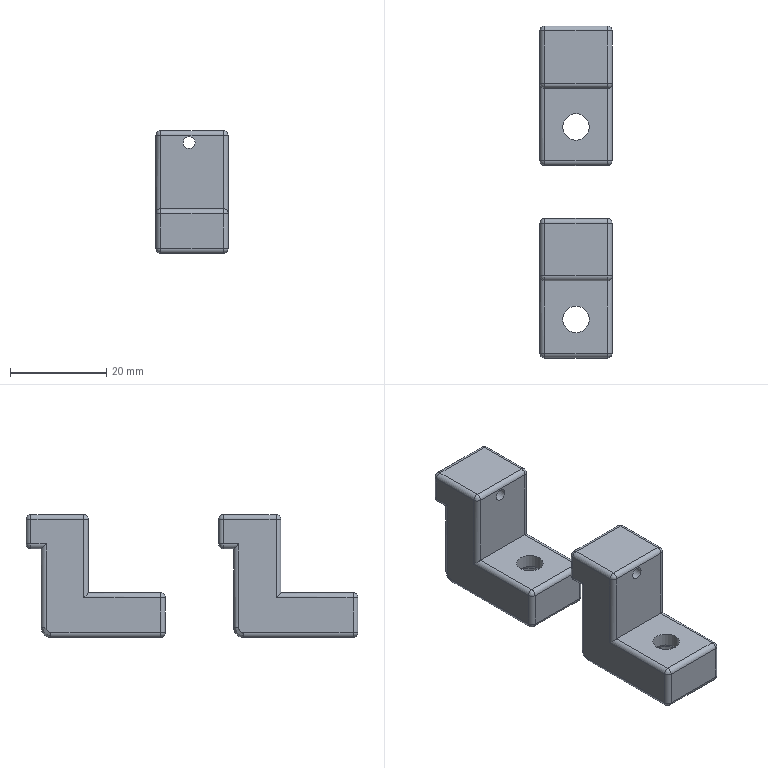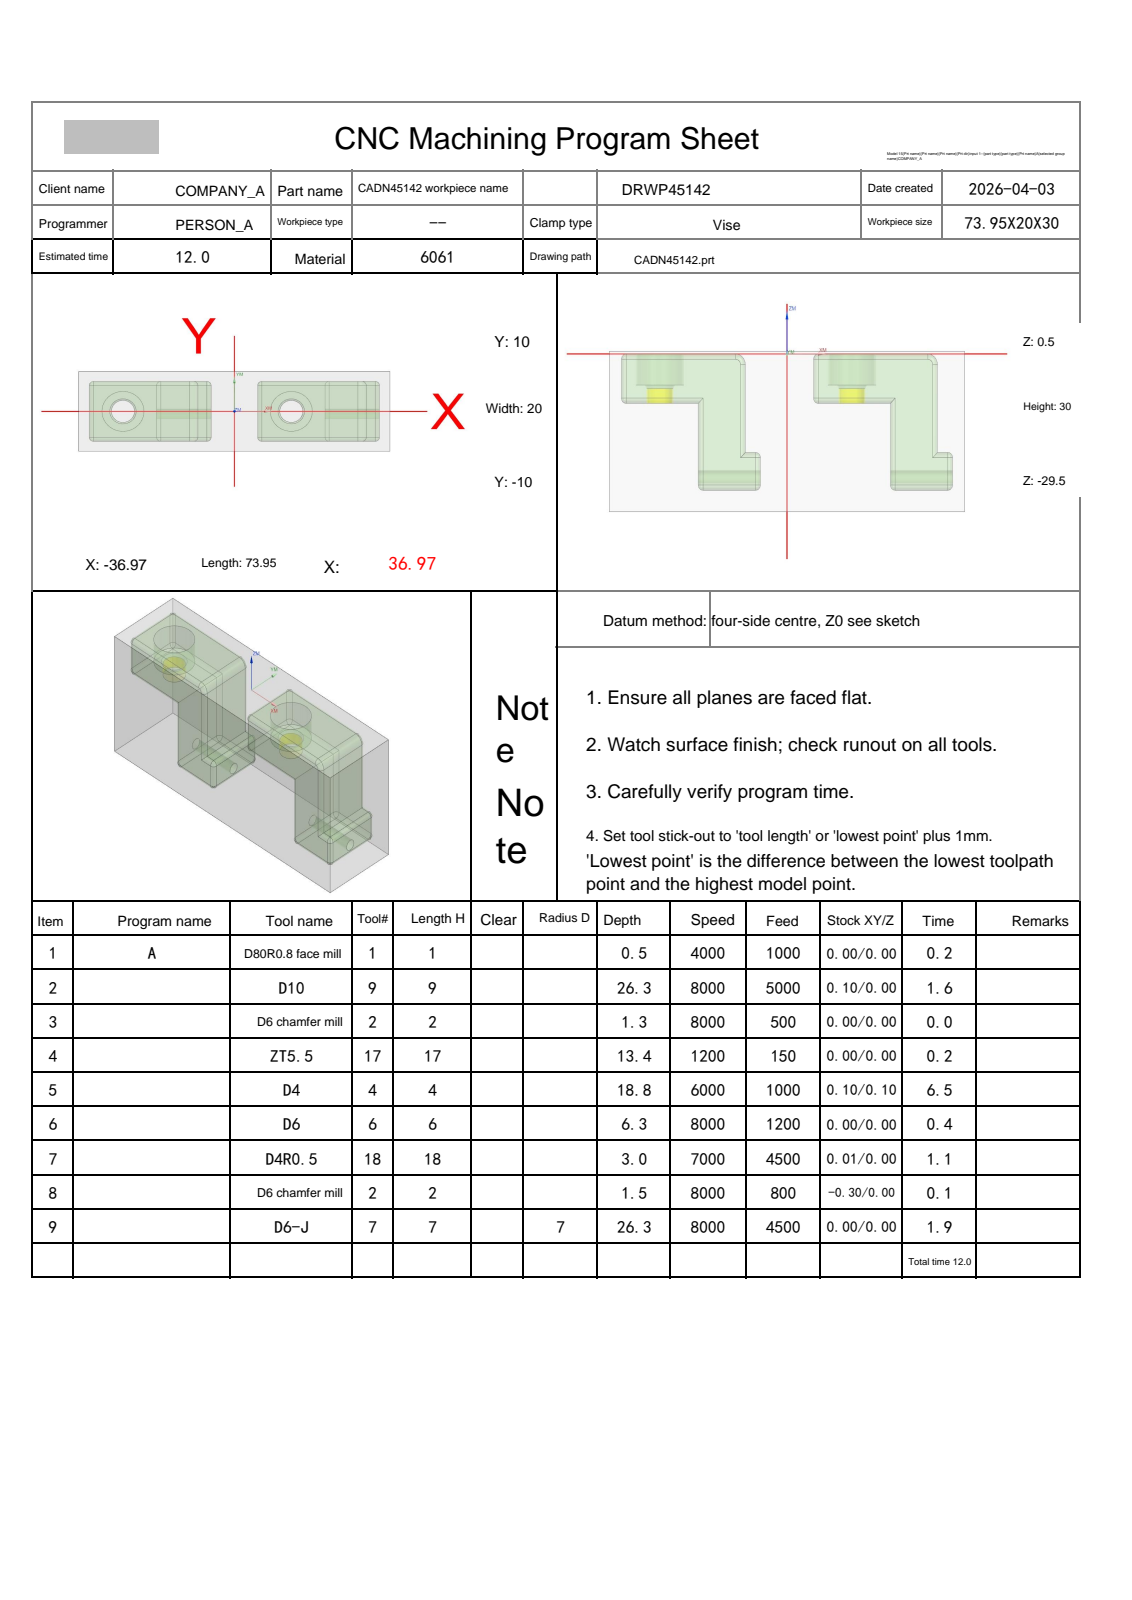NC program | NX | posted by the shop | part box 15 x 68.95 x 25.5 mm
Lines 1 to 3214 of 6074, first 2006 of 3212 lines:
%
O0001
(Machine time: 13.80 MIN)
(===Total Tool:8===)
(T1=D80R0.8 face mill D=80.  R=0.8  D-  H01 Z=-0.   )
(T9=D10     D=10.  R=0.   D-  H09 Z=-25.8 )
(T2=D6 chamfer mill   D=6.   R=0.   D-  H02 Z=-1.   )
(T17=ZT5.5  D=5.5  DR_a=118 D-  H17 Z=-12.9 )
(T4=D4      D=4.   R=0.   D-  H04 Z=-18.31)
(T6=D6      D=6.   R=0.   D6  H06 Z=-5.8  )
(T18=D4R0.5 D=4.   R=0.5  D-  H18 Z=-2.5  )
(T7=D6-J    D=6.   R=0.   D7  H07 Z=-25.8 )
G80 G90 G17 G49 G40
G91 G28 Z0
M01
N1 T01 M06
(D80R0.8 face mill D=80. R=0.8 H=01 ce=0.00 di=0.00)
G00 G90 G54 X-79.475 Y0.0 M03 S4000
G43 H01 Z20.
M08
Z2.
G01 Z0.0 F1000.
X-74.475
X74.475
X79.475
Z2.
G00 Z20.
G91 G28 Z0.0
M05
M09
G91 G28 Z0.0
M01
N2 T09 M06
(D10  D=10. R=0. H=09 ce=0.10 di=0.00)
G00 G90 G54 X20. Y-12.6 M03 S8000
G43 H09 Z20.
M08
Z.5
G01 X6.525 Z.409 F5000.
G02 X.425 Y-6.5 Z.345 I0.0 J6.1
G01 Y6.5 Z.257
G02 X6.525 Y12.6 Z.192 I6.1 J0.0
G01 X33.475 Z.011
G02 X39.575 Y6.5 Z-.054 I0.0 J-6.1
G01 Y-6.5 Z-.142
G02 X33.475 Y-12.6 Z-.206 I-6.1 J0.0
G01 X6.525 Z-.388
G02 X.425 Y-6.5 Z-.452 I0.0 J6.1
G01 Y6.5 Z-.54
G02 X6.525 Y12.6 Z-.605 I6.1 J0.0
G01 X33.475 Z-.786
G02 X39.575 Y6.5 Z-.851 I0.0 J-6.1
G01 Y-6.5 Z-.939
G02 X33.475 Y-12.6 Z-1.003 I-6.1 J0.0
G01 X6.525 Z-1.185
G02 X.425 Y-6.5 Z-1.249 I0.0 J6.1
G01 Y6.5 Z-1.337
G02 X6.525 Y12.6 Z-1.402 I6.1 J0.0
G01 X33.475 Z-1.583
G02 X39.575 Y6.5 Z-1.648 I0.0 J-6.1
G01 Y-6.5 Z-1.735
G02 X33.475 Y-12.6 Z-1.8 I-6.1 J0.0
G01 X6.525 Z-1.982
G02 X.425 Y-6.5 Z-2.046 I0.0 J6.1
G01 Y6.5 Z-2.134
G02 X6.525 Y12.6 Z-2.199 I6.1 J0.0
G01 X33.475 Z-2.38
G02 X39.575 Y6.5 Z-2.445 I0.0 J-6.1
G01 Y-6.5 Z-2.532
G02 X33.475 Y-12.6 Z-2.597 I-6.1 J0.0
G01 X6.525 Z-2.779
G02 X.425 Y-6.5 Z-2.843 I0.0 J6.1
G01 Y6.5 Z-2.931
G02 X6.525 Y12.6 Z-2.996 I6.1 J0.0
G01 X33.475 Z-3.177
G02 X39.575 Y6.5 Z-3.242 I0.0 J-6.1
G01 Y-6.5 Z-3.329
G02 X33.475 Y-12.6 Z-3.394 I-6.1 J0.0
G01 X6.525 Z-3.576
G02 X.425 Y-6.5 Z-3.64 I0.0 J6.1
G01 Y6.5 Z-3.728
G02 X6.525 Y12.6 Z-3.793 I6.1 J0.0
G01 X33.475 Z-3.974
G02 X39.575 Y6.5 Z-4.039 I0.0 J-6.1
G01 Y-6.5 Z-4.126
G02 X33.475 Y-12.6 Z-4.191 I-6.1 J0.0
G01 X6.525 Z-4.373
G02 X.425 Y-6.5 Z-4.437 I0.0 J6.1
G01 Y6.5 Z-4.525
G02 X6.525 Y12.6 Z-4.589 I6.1 J0.0
G01 X33.475 Z-4.771
G02 X39.575 Y6.5 Z-4.836 I0.0 J-6.1
G01 Y-6.5 Z-4.923
G02 X33.475 Y-12.6 Z-4.988 I-6.1 J0.0
G01 X6.525 Z-5.17
G02 X.425 Y-6.5 Z-5.234 I0.0 J6.1
G01 Y6.5 Z-5.322
G02 X6.525 Y12.6 Z-5.386 I6.1 J0.0
G01 X33.475 Z-5.568
G02 X39.575 Y6.5 Z-5.633 I0.0 J-6.1
G01 Y-6.5 Z-5.72
G02 X33.475 Y-12.6 Z-5.785 I-6.1 J0.0
G01 X6.525 Z-5.967
G02 X.425 Y-6.5 Z-6.031 I0.0 J6.1
G01 Y6.5 Z-6.119
G02 X6.525 Y12.6 Z-6.183 I6.1 J0.0
G01 X33.475 Z-6.365
G02 X39.575 Y6.5 Z-6.43 I0.0 J-6.1
G01 Y-6.5 Z-6.517
G02 X33.475 Y-12.6 Z-6.582 I-6.1 J0.0
G01 X6.525 Z-6.764
G02 X.425 Y-6.5 Z-6.828 I0.0 J6.1
G01 Y6.5 Z-6.916
G02 X6.525 Y12.6 Z-6.98 I6.1 J0.0
G01 X33.475 Z-7.162
G02 X39.575 Y6.5 Z-7.227 I0.0 J-6.1
G01 Y-6.5 Z-7.314
G02 X33.475 Y-12.6 Z-7.379 I-6.1 J0.0
G01 X6.525 Z-7.561
G02 X.425 Y-6.5 Z-7.625 I0.0 J6.1
G01 Y6.5 Z-7.713
G02 X6.525 Y12.6 Z-7.777 I6.1 J0.0
G01 X33.475 Z-7.959
G02 X39.575 Y6.5 Z-8.024 I0.0 J-6.1
G01 Y-6.5 Z-8.111
G02 X33.475 Y-12.6 Z-8.176 I-6.1 J0.0
G01 X6.525 Z-8.358
G02 X.425 Y-6.5 Z-8.422 I0.0 J6.1
G01 Y6.5 Z-8.51
G02 X6.525 Y12.6 Z-8.574 I6.1 J0.0
G01 X33.475 Z-8.756
G02 X39.575 Y6.5 Z-8.821 I0.0 J-6.1
G01 Y-6.5 Z-8.908
G02 X33.475 Y-12.6 Z-8.973 I-6.1 J0.0
G01 X6.525 Z-9.154
G02 X.425 Y-6.5 Z-9.219 I0.0 J6.1
G01 Y6.5 Z-9.307
G02 X6.525 Y12.6 Z-9.371 I6.1 J0.0
G01 X33.475 Z-9.553
G02 X39.575 Y6.5 Z-9.618 I0.0 J-6.1
G01 Y-6.5 Z-9.705
G02 X33.475 Y-12.6 Z-9.77 I-6.1 J0.0
G01 X6.525 Z-9.951
G02 X.425 Y-6.5 Z-10.016 I0.0 J6.1
G01 Y6.5 Z-10.104
G02 X6.525 Y12.6 Z-10.168 I6.1 J0.0
G01 X33.475 Z-10.35
G02 X39.575 Y6.5 Z-10.415 I0.0 J-6.1
G01 Y-6.5 Z-10.502
G02 X33.475 Y-12.6 Z-10.567 I-6.1 J0.0
G01 X6.525 Z-10.748
G02 X.425 Y-6.5 Z-10.813 I0.0 J6.1
G01 Y6.5 Z-10.901
G02 X6.525 Y12.6 Z-10.965 I6.1 J0.0
G01 X33.475 Z-11.147
G02 X39.575 Y6.5 Z-11.211 I0.0 J-6.1
G01 Y-6.5 Z-11.299
G02 X33.475 Y-12.6 Z-11.364 I-6.1 J0.0
G01 X6.525 Z-11.545
G02 X.425 Y-6.5 Z-11.61 I0.0 J6.1
G01 Y6.5 Z-11.698
G02 X6.525 Y12.6 Z-11.762 I6.1 J0.0
G01 X33.475 Z-11.944
G02 X39.575 Y6.5 Z-12.008 I0.0 J-6.1
G01 Y-6.5 Z-12.096
G02 X33.475 Y-12.6 Z-12.161 I-6.1 J0.0
G01 X6.525 Z-12.342
G02 X.425 Y-6.5 Z-12.407 I0.0 J6.1
G01 Y6.5 Z-12.495
G02 X6.525 Y12.6 Z-12.559 I6.1 J0.0
G01 X33.475 Z-12.741
G02 X39.575 Y6.5 Z-12.805 I0.0 J-6.1
G01 Y-6.5 Z-12.893
G02 X33.475 Y-12.6 Z-12.958 I-6.1 J0.0
G01 X6.525 Z-13.139
G02 X.425 Y-6.5 Z-13.204 I0.0 J6.1
G01 Y6.5 Z-13.292
G02 X6.525 Y12.6 Z-13.356 I6.1 J0.0
G01 X33.475 Z-13.538
G02 X39.575 Y6.5 Z-13.602 I0.0 J-6.1
G01 Y-6.5 Z-13.69
G02 X33.475 Y-12.6 Z-13.755 I-6.1 J0.0
G01 X6.525 Z-13.936
G02 X.425 Y-6.5 Z-14.001 I0.0 J6.1
G01 Y6.5 Z-14.089
G02 X6.525 Y12.6 Z-14.153 I6.1 J0.0
G01 X33.475 Z-14.335
G02 X39.575 Y6.5 Z-14.399 I0.0 J-6.1
G01 Y-6.5 Z-14.487
G02 X33.475 Y-12.6 Z-14.552 I-6.1 J0.0
G01 X6.525 Z-14.733
G02 X.425 Y-6.5 Z-14.798 I0.0 J6.1
G01 Y6.5 Z-14.885
G02 X6.525 Y12.6 Z-14.95 I6.1 J0.0
G01 X33.475 Z-15.132
G02 X39.575 Y6.5 Z-15.196 I0.0 J-6.1
G01 Y-6.5 Z-15.284
G02 X33.475 Y-12.6 Z-15.349 I-6.1 J0.0
G01 X6.525 Z-15.53
G02 X.425 Y-6.5 Z-15.595 I0.0 J6.1
G01 Y6.5 Z-15.682
G02 X6.525 Y12.6 Z-15.747 I6.1 J0.0
G01 X33.475 Z-15.929
G02 X39.575 Y6.5 Z-15.993 I0.0 J-6.1
G01 Y-6.5 Z-16.081
G02 X33.475 Y-12.6 Z-16.146 I-6.1 J0.0
G01 X6.525 Z-16.327
G02 X.425 Y-6.5 Z-16.392 I0.0 J6.1
G01 Y6.5 Z-16.479
G02 X6.525 Y12.6 Z-16.544 I6.1 J0.0
G01 X33.475 Z-16.726
G02 X39.575 Y6.5 Z-16.79 I0.0 J-6.1
G01 Y-6.5 Z-16.878
G02 X33.475 Y-12.6 Z-16.943 I-6.1 J0.0
G01 X6.525 Z-17.124
G02 X.425 Y-6.5 Z-17.189 I0.0 J6.1
G01 Y6.5 Z-17.276
G02 X6.525 Y12.6 Z-17.341 I6.1 J0.0
G01 X33.475 Z-17.523
G02 X39.575 Y6.5 Z-17.587 I0.0 J-6.1
G01 Y-6.5 Z-17.675
G02 X33.475 Y-12.6 Z-17.739 I-6.1 J0.0
G01 X6.525 Z-17.921
G02 X.425 Y-6.5 Z-17.986 I0.0 J6.1
G01 Y6.5 Z-18.073
G02 X6.525 Y12.6 Z-18.138 I6.1 J0.0
G01 X33.475 Z-18.32
G02 X39.575 Y6.5 Z-18.384 I0.0 J-6.1
G01 Y-6.5 Z-18.472
G02 X33.475 Y-12.6 Z-18.536 I-6.1 J0.0
G01 X6.525 Z-18.718
G02 X.425 Y-6.5 Z-18.783 I0.0 J6.1
G01 Y6.5 Z-18.87
G02 X6.525 Y12.6 Z-18.935 I6.1 J0.0
G01 X33.475 Z-19.117
G02 X39.575 Y6.5 Z-19.181 I0.0 J-6.1
G01 Y-6.5 Z-19.269
G02 X33.475 Y-12.6 Z-19.333 I-6.1 J0.0
G01 X6.525 Z-19.515
G02 X.425 Y-6.5 Z-19.58 I0.0 J6.1
G01 Y6.5 Z-19.667
G02 X6.525 Y12.6 Z-19.732 I6.1 J0.0
G01 X33.475 Z-19.914
G02 X39.575 Y6.5 Z-19.978 I0.0 J-6.1
G01 Y-6.5 Z-20.066
G02 X33.475 Y-12.6 Z-20.13 I-6.1 J0.0
G01 X6.525 Z-20.312
G02 X.425 Y-6.5 Z-20.377 I0.0 J6.1
G01 Y6.5 Z-20.464
G02 X6.525 Y12.6 Z-20.529 I6.1 J0.0
G01 X33.475 Z-20.711
G02 X39.575 Y6.5 Z-20.775 I0.0 J-6.1
G01 Y-6.5 Z-20.863
G02 X33.475 Y-12.6 Z-20.927 I-6.1 J0.0
G01 X6.525 Z-21.109
G02 X.425 Y-6.5 Z-21.174 I0.0 J6.1
G01 Y6.5 Z-21.261
G02 X6.525 Y12.6 Z-21.326 I6.1 J0.0
G01 X33.475 Z-21.508
G02 X39.575 Y6.5 Z-21.572 I0.0 J-6.1
G01 Y-6.5 Z-21.66
G02 X33.475 Y-12.6 Z-21.724 I-6.1 J0.0
G01 X6.525 Z-21.906
G02 X.425 Y-6.5 Z-21.971 I0.0 J6.1
G01 Y6.5 Z-22.058
G02 X6.525 Y12.6 Z-22.123 I6.1 J0.0
G01 X33.475 Z-22.304
G02 X39.575 Y6.5 Z-22.369 I0.0 J-6.1
G01 Y-6.5 Z-22.457
G02 X33.475 Y-12.6 Z-22.521 I-6.1 J0.0
G01 X6.525 Z-22.703
G02 X.425 Y-6.5 Z-22.768 I0.0 J6.1
G01 Y6.5 Z-22.855
G02 X6.525 Y12.6 Z-22.92 I6.1 J0.0
G01 X33.475 Z-23.101
G02 X39.575 Y6.5 Z-23.166 I0.0 J-6.1
G01 Y-6.5 Z-23.254
G02 X33.475 Y-12.6 Z-23.318 I-6.1 J0.0
G01 X6.525 Z-23.5
G02 X.425 Y-6.5 Z-23.565 I0.0 J6.1
G01 Y6.5 Z-23.652
G02 X6.525 Y12.6 Z-23.717 I6.1 J0.0
G01 X33.475 Z-23.898
G02 X39.575 Y6.5 Z-23.963 I0.0 J-6.1
G01 Y-6.5 Z-24.051
G02 X33.475 Y-12.6 Z-24.115 I-6.1 J0.0
G01 X6.525 Z-24.297
G02 X.425 Y-6.5 Z-24.361 I0.0 J6.1
G01 Y6.5 Z-24.449
G02 X6.525 Y12.6 Z-24.514 I6.1 J0.0
G01 X33.475 Z-24.695
G02 X39.575 Y6.5 Z-24.76 I0.0 J-6.1
G01 Y-6.5 Z-24.848
G02 X33.475 Y-12.6 Z-24.912 I-6.1 J0.0
G01 X6.525 Z-25.094
G02 X.425 Y-6.5 Z-25.158 I0.0 J6.1
G01 Y6.5 Z-25.246
G02 X6.525 Y12.6 Z-25.311 I6.1 J0.0
G01 X33.475 Z-25.492
G02 X39.575 Y6.5 Z-25.557 I0.0 J-6.1
G01 Y-6.5 Z-25.645
G02 X33.475 Y-12.6 Z-25.709 I-6.1 J0.0
G01 X20. Z-25.8
X6.525
G02 X.425 Y-6.5 I0.0 J6.1
G01 Y6.5
G02 X6.525 Y12.6 I6.1 J0.0
G01 X33.475
G02 X39.575 Y6.5 I0.0 J-6.1
G01 Y-6.5
G02 X33.475 Y-12.6 I-6.1 J0.0
G01 X20.
X19.5
Z-24.8
G00 Z20.
X-20.
Z.5
G01 X-33.475 Z.409
G02 X-39.575 Y-6.5 Z.345 I0.0 J6.1
G01 Y6.5 Z.257
G02 X-33.475 Y12.6 Z.192 I6.1 J0.0
G01 X-6.525 Z.011
G02 X-.425 Y6.5 Z-.054 I0.0 J-6.1
G01 Y-6.5 Z-.142
G02 X-6.525 Y-12.6 Z-.206 I-6.1 J0.0
G01 X-33.475 Z-.388
G02 X-39.575 Y-6.5 Z-.452 I0.0 J6.1
G01 Y6.5 Z-.54
G02 X-33.475 Y12.6 Z-.605 I6.1 J0.0
G01 X-6.525 Z-.786
G02 X-.425 Y6.5 Z-.851 I0.0 J-6.1
G01 Y-6.5 Z-.939
G02 X-6.525 Y-12.6 Z-1.003 I-6.1 J0.0
G01 X-33.475 Z-1.185
G02 X-39.575 Y-6.5 Z-1.249 I0.0 J6.1
G01 Y6.5 Z-1.337
G02 X-33.475 Y12.6 Z-1.402 I6.1 J0.0
G01 X-6.525 Z-1.583
G02 X-.425 Y6.5 Z-1.648 I0.0 J-6.1
G01 Y-6.5 Z-1.735
G02 X-6.525 Y-12.6 Z-1.8 I-6.1 J0.0
G01 X-33.475 Z-1.982
G02 X-39.575 Y-6.5 Z-2.046 I0.0 J6.1
G01 Y6.5 Z-2.134
G02 X-33.475 Y12.6 Z-2.199 I6.1 J0.0
G01 X-6.525 Z-2.38
G02 X-.425 Y6.5 Z-2.445 I0.0 J-6.1
G01 Y-6.5 Z-2.532
G02 X-6.525 Y-12.6 Z-2.597 I-6.1 J0.0
G01 X-33.475 Z-2.779
G02 X-39.575 Y-6.5 Z-2.843 I0.0 J6.1
G01 Y6.5 Z-2.931
G02 X-33.475 Y12.6 Z-2.996 I6.1 J0.0
G01 X-6.525 Z-3.177
G02 X-.425 Y6.5 Z-3.242 I0.0 J-6.1
G01 Y-6.5 Z-3.329
G02 X-6.525 Y-12.6 Z-3.394 I-6.1 J0.0
G01 X-33.475 Z-3.576
G02 X-39.575 Y-6.5 Z-3.64 I0.0 J6.1
G01 Y6.5 Z-3.728
G02 X-33.475 Y12.6 Z-3.793 I6.1 J0.0
G01 X-6.525 Z-3.974
G02 X-.425 Y6.5 Z-4.039 I0.0 J-6.1
G01 Y-6.5 Z-4.126
G02 X-6.525 Y-12.6 Z-4.191 I-6.1 J0.0
G01 X-33.475 Z-4.373
G02 X-39.575 Y-6.5 Z-4.437 I0.0 J6.1
G01 Y6.5 Z-4.525
G02 X-33.475 Y12.6 Z-4.589 I6.1 J0.0
G01 X-6.525 Z-4.771
G02 X-.425 Y6.5 Z-4.836 I0.0 J-6.1
G01 Y-6.5 Z-4.923
G02 X-6.525 Y-12.6 Z-4.988 I-6.1 J0.0
G01 X-33.475 Z-5.17
G02 X-39.575 Y-6.5 Z-5.234 I0.0 J6.1
G01 Y6.5 Z-5.322
G02 X-33.475 Y12.6 Z-5.386 I6.1 J0.0
G01 X-6.525 Z-5.568
G02 X-.425 Y6.5 Z-5.633 I0.0 J-6.1
G01 Y-6.5 Z-5.72
G02 X-6.525 Y-12.6 Z-5.785 I-6.1 J0.0
G01 X-33.475 Z-5.967
G02 X-39.575 Y-6.5 Z-6.031 I0.0 J6.1
G01 Y6.5 Z-6.119
G02 X-33.475 Y12.6 Z-6.183 I6.1 J0.0
G01 X-6.525 Z-6.365
G02 X-.425 Y6.5 Z-6.43 I0.0 J-6.1
G01 Y-6.5 Z-6.517
G02 X-6.525 Y-12.6 Z-6.582 I-6.1 J0.0
G01 X-33.475 Z-6.764
G02 X-39.575 Y-6.5 Z-6.828 I0.0 J6.1
G01 Y6.5 Z-6.916
G02 X-33.475 Y12.6 Z-6.98 I6.1 J0.0
G01 X-6.525 Z-7.162
G02 X-.425 Y6.5 Z-7.227 I0.0 J-6.1
G01 Y-6.5 Z-7.314
G02 X-6.525 Y-12.6 Z-7.379 I-6.1 J0.0
G01 X-33.475 Z-7.561
G02 X-39.575 Y-6.5 Z-7.625 I0.0 J6.1
G01 Y6.5 Z-7.713
G02 X-33.475 Y12.6 Z-7.777 I6.1 J0.0
G01 X-6.525 Z-7.959
G02 X-.425 Y6.5 Z-8.024 I0.0 J-6.1
G01 Y-6.5 Z-8.111
G02 X-6.525 Y-12.6 Z-8.176 I-6.1 J0.0
G01 X-33.475 Z-8.358
G02 X-39.575 Y-6.5 Z-8.422 I0.0 J6.1
G01 Y6.5 Z-8.51
G02 X-33.475 Y12.6 Z-8.574 I6.1 J0.0
G01 X-6.525 Z-8.756
G02 X-.425 Y6.5 Z-8.821 I0.0 J-6.1
G01 Y-6.5 Z-8.908
G02 X-6.525 Y-12.6 Z-8.973 I-6.1 J0.0
G01 X-33.475 Z-9.154
G02 X-39.575 Y-6.5 Z-9.219 I0.0 J6.1
G01 Y6.5 Z-9.307
G02 X-33.475 Y12.6 Z-9.371 I6.1 J0.0
G01 X-6.525 Z-9.553
G02 X-.425 Y6.5 Z-9.618 I0.0 J-6.1
G01 Y-6.5 Z-9.705
G02 X-6.525 Y-12.6 Z-9.77 I-6.1 J0.0
G01 X-33.475 Z-9.951
G02 X-39.575 Y-6.5 Z-10.016 I0.0 J6.1
G01 Y6.5 Z-10.104
G02 X-33.475 Y12.6 Z-10.168 I6.1 J0.0
G01 X-6.525 Z-10.35
G02 X-.425 Y6.5 Z-10.415 I0.0 J-6.1
G01 Y-6.5 Z-10.502
G02 X-6.525 Y-12.6 Z-10.567 I-6.1 J0.0
G01 X-33.475 Z-10.748
G02 X-39.575 Y-6.5 Z-10.813 I0.0 J6.1
G01 Y6.5 Z-10.901
G02 X-33.475 Y12.6 Z-10.965 I6.1 J0.0
G01 X-6.525 Z-11.147
G02 X-.425 Y6.5 Z-11.211 I0.0 J-6.1
G01 Y-6.5 Z-11.299
G02 X-6.525 Y-12.6 Z-11.364 I-6.1 J0.0
G01 X-33.475 Z-11.545
G02 X-39.575 Y-6.5 Z-11.61 I0.0 J6.1
G01 Y6.5 Z-11.698
G02 X-33.475 Y12.6 Z-11.762 I6.1 J0.0
G01 X-6.525 Z-11.944
G02 X-.425 Y6.5 Z-12.008 I0.0 J-6.1
G01 Y-6.5 Z-12.096
G02 X-6.525 Y-12.6 Z-12.161 I-6.1 J0.0
G01 X-33.475 Z-12.342
G02 X-39.575 Y-6.5 Z-12.407 I0.0 J6.1
G01 Y6.5 Z-12.495
G02 X-33.475 Y12.6 Z-12.559 I6.1 J0.0
G01 X-6.525 Z-12.741
G02 X-.425 Y6.5 Z-12.805 I0.0 J-6.1
G01 Y-6.5 Z-12.893
G02 X-6.525 Y-12.6 Z-12.958 I-6.1 J0.0
G01 X-33.475 Z-13.139
G02 X-39.575 Y-6.5 Z-13.204 I0.0 J6.1
G01 Y6.5 Z-13.292
G02 X-33.475 Y12.6 Z-13.356 I6.1 J0.0
G01 X-6.525 Z-13.538
G02 X-.425 Y6.5 Z-13.602 I0.0 J-6.1
G01 Y-6.5 Z-13.69
G02 X-6.525 Y-12.6 Z-13.755 I-6.1 J0.0
G01 X-33.475 Z-13.936
G02 X-39.575 Y-6.5 Z-14.001 I0.0 J6.1
G01 Y6.5 Z-14.089
G02 X-33.475 Y12.6 Z-14.153 I6.1 J0.0
G01 X-6.525 Z-14.335
G02 X-.425 Y6.5 Z-14.399 I0.0 J-6.1
G01 Y-6.5 Z-14.487
G02 X-6.525 Y-12.6 Z-14.552 I-6.1 J0.0
G01 X-33.475 Z-14.733
G02 X-39.575 Y-6.5 Z-14.798 I0.0 J6.1
G01 Y6.5 Z-14.885
G02 X-33.475 Y12.6 Z-14.95 I6.1 J0.0
G01 X-6.525 Z-15.132
G02 X-.425 Y6.5 Z-15.196 I0.0 J-6.1
G01 Y-6.5 Z-15.284
G02 X-6.525 Y-12.6 Z-15.349 I-6.1 J0.0
G01 X-33.475 Z-15.53
G02 X-39.575 Y-6.5 Z-15.595 I0.0 J6.1
G01 Y6.5 Z-15.682
G02 X-33.475 Y12.6 Z-15.747 I6.1 J0.0
G01 X-6.525 Z-15.929
G02 X-.425 Y6.5 Z-15.993 I0.0 J-6.1
G01 Y-6.5 Z-16.081
G02 X-6.525 Y-12.6 Z-16.146 I-6.1 J0.0
G01 X-33.475 Z-16.327
G02 X-39.575 Y-6.5 Z-16.392 I0.0 J6.1
G01 Y6.5 Z-16.479
G02 X-33.475 Y12.6 Z-16.544 I6.1 J0.0
G01 X-6.525 Z-16.726
G02 X-.425 Y6.5 Z-16.79 I0.0 J-6.1
G01 Y-6.5 Z-16.878
G02 X-6.525 Y-12.6 Z-16.943 I-6.1 J0.0
G01 X-33.475 Z-17.124
G02 X-39.575 Y-6.5 Z-17.189 I0.0 J6.1
G01 Y6.5 Z-17.276
G02 X-33.475 Y12.6 Z-17.341 I6.1 J0.0
G01 X-6.525 Z-17.523
G02 X-.425 Y6.5 Z-17.587 I0.0 J-6.1
G01 Y-6.5 Z-17.675
G02 X-6.525 Y-12.6 Z-17.739 I-6.1 J0.0
G01 X-33.475 Z-17.921
G02 X-39.575 Y-6.5 Z-17.986 I0.0 J6.1
G01 Y6.5 Z-18.073
G02 X-33.475 Y12.6 Z-18.138 I6.1 J0.0
G01 X-6.525 Z-18.32
G02 X-.425 Y6.5 Z-18.384 I0.0 J-6.1
G01 Y-6.5 Z-18.472
G02 X-6.525 Y-12.6 Z-18.536 I-6.1 J0.0
G01 X-33.475 Z-18.718
G02 X-39.575 Y-6.5 Z-18.783 I0.0 J6.1
G01 Y6.5 Z-18.87
G02 X-33.475 Y12.6 Z-18.935 I6.1 J0.0
G01 X-6.525 Z-19.117
G02 X-.425 Y6.5 Z-19.181 I0.0 J-6.1
G01 Y-6.5 Z-19.269
G02 X-6.525 Y-12.6 Z-19.333 I-6.1 J0.0
G01 X-33.475 Z-19.515
G02 X-39.575 Y-6.5 Z-19.58 I0.0 J6.1
G01 Y6.5 Z-19.667
G02 X-33.475 Y12.6 Z-19.732 I6.1 J0.0
G01 X-6.525 Z-19.914
G02 X-.425 Y6.5 Z-19.978 I0.0 J-6.1
G01 Y-6.5 Z-20.066
G02 X-6.525 Y-12.6 Z-20.13 I-6.1 J0.0
G01 X-33.475 Z-20.312
G02 X-39.575 Y-6.5 Z-20.377 I0.0 J6.1
G01 Y6.5 Z-20.464
G02 X-33.475 Y12.6 Z-20.529 I6.1 J0.0
G01 X-6.525 Z-20.711
G02 X-.425 Y6.5 Z-20.775 I0.0 J-6.1
G01 Y-6.5 Z-20.863
G02 X-6.525 Y-12.6 Z-20.927 I-6.1 J0.0
G01 X-33.475 Z-21.109
G02 X-39.575 Y-6.5 Z-21.174 I0.0 J6.1
G01 Y6.5 Z-21.261
G02 X-33.475 Y12.6 Z-21.326 I6.1 J0.0
G01 X-6.525 Z-21.508
G02 X-.425 Y6.5 Z-21.572 I0.0 J-6.1
G01 Y-6.5 Z-21.66
G02 X-6.525 Y-12.6 Z-21.724 I-6.1 J0.0
G01 X-33.475 Z-21.906
G02 X-39.575 Y-6.5 Z-21.971 I0.0 J6.1
G01 Y6.5 Z-22.058
G02 X-33.475 Y12.6 Z-22.123 I6.1 J0.0
G01 X-6.525 Z-22.304
G02 X-.425 Y6.5 Z-22.369 I0.0 J-6.1
G01 Y-6.5 Z-22.457
G02 X-6.525 Y-12.6 Z-22.521 I-6.1 J0.0
G01 X-33.475 Z-22.703
G02 X-39.575 Y-6.5 Z-22.768 I0.0 J6.1
G01 Y6.5 Z-22.855
G02 X-33.475 Y12.6 Z-22.92 I6.1 J0.0
G01 X-6.525 Z-23.101
G02 X-.425 Y6.5 Z-23.166 I0.0 J-6.1
G01 Y-6.5 Z-23.254
G02 X-6.525 Y-12.6 Z-23.318 I-6.1 J0.0
G01 X-33.475 Z-23.5
G02 X-39.575 Y-6.5 Z-23.565 I0.0 J6.1
G01 Y6.5 Z-23.652
G02 X-33.475 Y12.6 Z-23.717 I6.1 J0.0
G01 X-6.525 Z-23.898
G02 X-.425 Y6.5 Z-23.963 I0.0 J-6.1
G01 Y-6.5 Z-24.051
G02 X-6.525 Y-12.6 Z-24.115 I-6.1 J0.0
G01 X-33.475 Z-24.297
G02 X-39.575 Y-6.5 Z-24.361 I0.0 J6.1
G01 Y6.5 Z-24.449
G02 X-33.475 Y12.6 Z-24.514 I6.1 J0.0
G01 X-6.525 Z-24.695
G02 X-.425 Y6.5 Z-24.76 I0.0 J-6.1
G01 Y-6.5 Z-24.848
G02 X-6.525 Y-12.6 Z-24.912 I-6.1 J0.0
G01 X-33.475 Z-25.094
G02 X-39.575 Y-6.5 Z-25.158 I0.0 J6.1
G01 Y6.5 Z-25.246
G02 X-33.475 Y12.6 Z-25.311 I6.1 J0.0
G01 X-6.525 Z-25.492
G02 X-.425 Y6.5 Z-25.557 I0.0 J-6.1
G01 Y-6.5 Z-25.645
G02 X-6.525 Y-12.6 Z-25.709 I-6.1 J0.0
G01 X-20. Z-25.8
X-33.475
G02 X-39.575 Y-6.5 I0.0 J6.1
G01 Y6.5
G02 X-33.475 Y12.6 I6.1 J0.0
G01 X-6.525
G02 X-.425 Y6.5 I0.0 J-6.1
G01 Y-6.5
G02 X-6.525 Y-12.6 I-6.1 J0.0
G01 X-20.
X-20.5
Z-24.8
G00 Z20.
G91 G28 Z0.0
M05
M09
G91 G28 Z0.0
M01
N3 T02 M06
(D6 chamfer mill  D=6. R=0. H=02 ce=0.00 di=0.00)
G00 G90 G54 X-26.475 Y0.0 M03 S8000
G43 H02 Z20.
M08
G98 G81 X-26.475 Y0.0 Z-.8 R1. F500.
X13.525
G80
G00 Z20.
G91 G28 Z0.0
M05
M09
G91 G28 Z0.0
M01
N4 T17 M06
(ZT5.5 D=5.5 DR_a=118 H=17)
G00 G90 G54 X-26.475 Y0.0 M03 S1200
G43 H17 Z20.
M08
G98 G83 X-26.475 Y0.0 Z-12.902 R1. F150. Q2.
X13.525
G80
G00 Z20.
G91 G28 Z0.0
M05
M09
G91 G28 Z0.0
M01
N5 T04 M06
(D4  D=4. R=0. H=04 ce=0.10 di=0.10)
G00 G90 G54 X38.475 Y0.0 M03 S6000
G43 H04 Z20.
M08
Z.301
G01 Z-.199 F1000.
X33.875
Y6.9
X33.4
G02 X33.425 Y6.5 I-3.074 J-.4
G01 X33.426 Y-6.5
G02 X33.4 Y-6.9 I-3.1 J0.0
G01 X33.875
Y0.0
Y.5
Z.301
G00 Z.5
X38.475 Y0.0
Z.102
G01 Z-.398
X33.875
Y6.9
X33.4
G02 X33.425 Y6.5 I-3.074 J-.4
G01 X33.426 Y-6.5
G02 X33.4 Y-6.9 I-3.1 J0.0
G01 X33.875
Y0.0
Y.5
Z.102
G00 Z.301
X38.475 Y0.0
Z-.097
G01 Z-.597
X33.875
Y6.9
X33.4
G02 X33.425 Y6.5 I-3.074 J-.4
G01 X33.426 Y-6.5
G02 X33.4 Y-6.9 I-3.1 J0.0
G01 X33.875
Y0.0
Y.5
Z-.097
G00 Z.102
X38.475 Y0.0
Z-.296
G01 Z-.796
X33.875
Y6.9
X33.4
G02 X33.425 Y6.5 I-3.074 J-.4
G01 X33.426 Y-6.5
G02 X33.4 Y-6.9 I-3.1 J0.0
G01 X33.875
Y0.0
Y.5
Z-.296
G00 Z-.097
X38.475 Y0.0
Z-.495
G01 Z-.995
X33.875
Y6.9
X33.4
G02 X33.425 Y6.5 I-3.074 J-.4
G01 X33.426 Y-6.5
G02 X33.4 Y-6.9 I-3.1 J0.0
G01 X33.875
Y0.0
Y.5
Z-.495
G00 Z-.296
X38.475 Y0.0
Z-.694
G01 Z-1.194
X33.875
Y6.9
X33.4
G02 X33.425 Y6.5 I-3.074 J-.4
G01 X33.426 Y-6.5
G02 X33.4 Y-6.9 I-3.1 J0.0
G01 X33.875
Y0.0
Y.5
Z-.694
G00 Z-.495
X38.475 Y0.0
Z-.893
G01 Z-1.393
X33.875
Y6.9
X33.4
G02 X33.425 Y6.5 I-3.074 J-.4
G01 X33.426 Y-6.5
G02 X33.4 Y-6.9 I-3.1 J0.0
G01 X33.875
Y0.0
Y.5
Z-.893
G00 Z-.694
X38.475 Y0.0
Z-1.092
G01 Z-1.592
X33.875
Y6.9
X33.4
G02 X33.425 Y6.5 I-3.074 J-.4
G01 X33.426 Y-6.5
G02 X33.4 Y-6.9 I-3.1 J0.0
G01 X33.875
Y0.0
Y.5
Z-1.092
G00 Z-.893
X38.475 Y0.0
Z-1.292
G01 Z-1.792
X33.875
Y6.9
X33.4
G02 X33.425 Y6.5 I-3.074 J-.4
G01 X33.426 Y-6.5
G02 X33.4 Y-6.9 I-3.1 J0.0
G01 X33.875
Y0.0
Y.5
Z-1.292
G00 Z-1.092
X38.475 Y0.0
Z-1.491
G01 Z-1.991
X33.875
Y6.9
X33.4
G02 X33.425 Y6.5 I-3.074 J-.4
G01 X33.426 Y-6.5
G02 X33.4 Y-6.9 I-3.1 J0.0
G01 X33.875
Y0.0
Y.5
Z-1.491
G00 Z-1.292
X38.475 Y0.0
Z-1.69
G01 Z-2.19
X33.875
Y6.9
X33.4
G02 X33.425 Y6.5 I-3.074 J-.4
G01 X33.426 Y-6.5
G02 X33.4 Y-6.9 I-3.1 J0.0
G01 X33.875
Y0.0
Y.5
Z-1.69
G00 Z-1.491
X38.475 Y0.0
Z-1.889
G01 Z-2.389
X33.875
Y6.9
X33.4
G02 X33.425 Y6.5 I-3.074 J-.4
G01 X33.426 Y-6.5
G02 X33.4 Y-6.9 I-3.1 J0.0
G01 X33.875
Y0.0
Y.5
Z-1.889
G00 Z-1.69
X38.475 Y0.0
Z-2.088
G01 Z-2.588
X33.875
Y6.9
X33.4
G02 X33.425 Y6.5 I-3.074 J-.4
G01 X33.426 Y-6.5
G02 X33.4 Y-6.9 I-3.1 J0.0
G01 X33.875
Y0.0
Y.5
Z-2.088
G00 Z-1.889
X38.475 Y0.0
Z-2.287
G01 Z-2.787
X33.875
Y6.9
X33.4
G02 X33.425 Y6.5 I-3.074 J-.4
G01 X33.426 Y-6.5
G02 X33.4 Y-6.9 I-3.1 J0.0
G01 X33.875
Y0.0
Y.5
Z-2.287
G00 Z-2.088
X38.475 Y0.0
Z-2.486
G01 Z-2.986
X33.875
Y6.9
X33.4
G02 X33.425 Y6.5 I-3.074 J-.4
G01 X33.426 Y-6.5
G02 X33.4 Y-6.9 I-3.1 J0.0
G01 X33.875
Y0.0
Y.5
Z-2.486
G00 Z-2.287
X38.475 Y0.0
Z-2.685
G01 Z-3.185
X33.875
Y6.9
X33.4
G02 X33.425 Y6.5 I-3.074 J-.4
G01 X33.426 Y-6.5
G02 X33.4 Y-6.9 I-3.1 J0.0
G01 X33.875
Y0.0
Y.5
Z-2.685
G00 Z-2.486
X38.475 Y0.0
Z-2.884
G01 Z-3.384
X33.875
Y6.9
X33.4
G02 X33.425 Y6.5 I-3.074 J-.4
G01 X33.426 Y-6.5
G02 X33.4 Y-6.9 I-3.1 J0.0
G01 X33.875
Y0.0
Y.5
Z-2.884
G00 Z-2.685
X38.475 Y0.0
Z-3.083
G01 Z-3.583
X33.875
Y6.9
X33.4
G02 X33.425 Y6.5 I-3.074 J-.4
G01 X33.426 Y-6.5
G02 X33.4 Y-6.9 I-3.1 J0.0
G01 X33.875
Y0.0
Y.5
Z-3.083
G00 Z-2.884
X38.475 Y0.0
Z-3.282
G01 Z-3.782
X33.875
Y6.9
X33.4
G02 X33.425 Y6.5 I-3.074 J-.4
G01 X33.426 Y-6.5
G02 X33.4 Y-6.9 I-3.1 J0.0
G01 X33.875
Y0.0
Y.5
Z-3.282
G00 Z-3.083
X38.475 Y0.0
Z-3.481
G01 Z-3.981
X33.875
Y6.9
X33.4
G02 X33.425 Y6.5 I-3.074 J-.4
G01 X33.426 Y-6.5
G02 X33.4 Y-6.9 I-3.1 J0.0
G01 X33.875
Y0.0
Y.5
Z-3.481
G00 Z-3.282
X38.475 Y0.0
Z-3.68
G01 Z-4.18
X33.875
Y6.9
X33.4
G02 X33.425 Y6.5 I-3.074 J-.4
G01 X33.426 Y-6.5
G02 X33.4 Y-6.9 I-3.1 J0.0
G01 X33.875
Y0.0
Y.5
Z-3.68
G00 Z-3.481
X38.475 Y0.0
Z-3.879
G01 Z-4.379
X33.875
Y6.9
X33.4
G02 X33.425 Y6.5 I-3.074 J-.4
G01 X33.426 Y-6.5
G02 X33.4 Y-6.9 I-3.1 J0.0
G01 X33.875
Y0.0
Y.5
Z-3.879
G00 Z-3.68
X38.475 Y0.0
Z-4.078
G01 Z-4.578
X33.875
Y6.9
X33.4
G02 X33.425 Y6.5 I-3.074 J-.4
G01 X33.426 Y-6.5
G02 X33.4 Y-6.9 I-3.1 J0.0
G01 X33.875
Y0.0
Y.5
Z-4.078
G00 Z-3.879
X38.475 Y0.0
Z-4.277
G01 Z-4.777
X33.875
Y6.9
X33.4
G02 X33.425 Y6.5 I-3.074 J-.4
G01 X33.426 Y-6.5
G02 X33.4 Y-6.9 I-3.1 J0.0
G01 X33.875
Y0.0
Y.5
Z-4.277
G00 Z-4.078
X38.475 Y0.0
Z-4.476
G01 Z-4.976
X33.875
Y6.9
X33.4
G02 X33.425 Y6.5 I-3.074 J-.4
G01 X33.426 Y-6.5
G02 X33.4 Y-6.9 I-3.1 J0.0
G01 X33.875
Y0.0
Y.5
Z-4.476
G00 Z-4.277
X38.475 Y0.0
Z-4.675
G01 Z-5.175
X33.875
Y6.9
X33.4
G02 X33.425 Y6.5 I-3.074 J-.4
G01 X33.426 Y-6.5
G02 X33.4 Y-6.9 I-3.1 J0.0
G01 X33.875
Y0.0
Y.5
Z-4.675
G00 Z-4.476
X38.475 Y0.0
Z-4.875
G01 Z-5.375
X33.875
Y6.9
X33.4
G02 X33.425 Y6.5 I-3.074 J-.4
G01 X33.426 Y-6.5
G02 X33.4 Y-6.9 I-3.1 J0.0
G01 X33.875
Y0.0
Y.5
Z-4.875
G00 Z-4.675
X38.475 Y0.0
Z-5.074
G01 Z-5.574
X33.875
Y6.9
X33.4
G02 X33.425 Y6.5 I-3.074 J-.4
G01 X33.426 Y-6.5
G02 X33.4 Y-6.9 I-3.1 J0.0
G01 X33.875
Y0.0
Y.5
Z-5.074
G00 Z-4.875
X38.475 Y0.0
Z-5.273
G01 Z-5.773
X33.875
Y6.9
X33.4
G02 X33.425 Y6.5 I-3.074 J-.4
G01 X33.426 Y-6.5
G02 X33.4 Y-6.9 I-3.1 J0.0
G01 X33.875
Y0.0
Y.5
Z-5.273
G00 Z-5.074
X38.475 Y0.0
Z-5.472
G01 Z-5.972
X33.875
Y6.9
X33.4
G02 X33.425 Y6.5 I-3.074 J-.4
G01 X33.426 Y-6.5
G02 X33.4 Y-6.9 I-3.1 J0.0
G01 X33.875
Y0.0
Y.5
Z-5.472
G00 Z-5.273
X38.475 Y0.0
Z-5.671
G01 Z-6.171
X33.875
Y6.9
X33.4
G02 X33.425 Y6.5 I-3.074 J-.4
G01 X33.426 Y-6.5
G02 X33.4 Y-6.9 I-3.1 J0.0
G01 X33.875
Y0.0
Y.5
Z-5.671
G00 Z-5.472
X38.475 Y0.0
Z-5.87
G01 Z-6.37
X33.875
Y6.9
X33.4
G02 X33.425 Y6.5 I-3.074 J-.4
G01 X33.426 Y-6.5
G02 X33.4 Y-6.9 I-3.1 J0.0
G01 X33.875
Y0.0
Y.5
Z-5.87
G00 Z-5.671
X38.475 Y0.0
Z-6.069
G01 Z-6.569
X33.875
Y6.9
X33.4
G02 X33.425 Y6.5 I-3.074 J-.4
G01 X33.426 Y-6.5
G02 X33.4 Y-6.9 I-3.1 J0.0
G01 X33.875
Y0.0
Y.5
Z-6.069
G00 Z-5.87
X38.475 Y0.0
Z-6.268
G01 Z-6.768
X33.875
Y6.9
X33.4
G02 X33.425 Y6.5 I-3.074 J-.4
G01 X33.426 Y-6.5
G02 X33.4 Y-6.9 I-3.1 J0.0
G01 X33.875
Y0.0
Y.5
Z-6.268
G00 Z-6.069
X38.475 Y0.0
Z-6.467
G01 Z-6.967
X33.875
Y6.9
X33.4
G02 X33.425 Y6.5 I-3.074 J-.4
G01 X33.426 Y-6.5
G02 X33.4 Y-6.9 I-3.1 J0.0
G01 X33.875
Y0.0
Y.5
Z-6.467
G00 Z-6.268
X38.475 Y0.0
Z-6.666
G01 Z-7.166
X33.875
Y6.9
X33.4
G02 X33.425 Y6.5 I-3.074 J-.4
G01 X33.426 Y-6.5
G02 X33.4 Y-6.9 I-3.1 J0.0
G01 X33.875
Y0.0
Y.5
Z-6.666
G00 Z-6.467
X38.475 Y0.0
Z-6.865
G01 Z-7.365
X33.875
Y6.9
X33.4
G02 X33.425 Y6.5 I-3.074 J-.4
G01 X33.426 Y-6.5
G02 X33.4 Y-6.9 I-3.1 J0.0
G01 X33.875
Y0.0
Y.5
Z-6.865
G00 Z-6.666
X38.475 Y0.0
Z-7.064
G01 Z-7.564
X33.875
Y6.9
X33.4
G02 X33.425 Y6.5 I-3.074 J-.4
G01 X33.426 Y-6.5
G02 X33.4 Y-6.9 I-3.1 J0.0
G01 X33.875
Y0.0
Y.5
Z-7.064
G00 Z-6.865
X38.475 Y0.0
Z-7.263
G01 Z-7.763
X33.875
Y6.9
X33.4
G02 X33.425 Y6.5 I-3.074 J-.4
G01 X33.426 Y-6.5
G02 X33.4 Y-6.9 I-3.1 J0.0
G01 X33.875
Y0.0
Y.5
Z-7.263
G00 Z-7.064
X38.475 Y0.0
Z-7.462
G01 Z-7.962
X33.875
Y6.9
X33.4
G02 X33.425 Y6.5 I-3.074 J-.4
G01 X33.426 Y-6.5
G02 X33.4 Y-6.9 I-3.1 J0.0
G01 X33.875
Y0.0
Y.5
Z-7.462
G00 Z-7.263
X38.475 Y0.0
Z-7.661
G01 Z-8.161
X33.875
Y6.9
X33.4
G02 X33.425 Y6.5 I-3.074 J-.4
G01 X33.426 Y-6.5
G02 X33.4 Y-6.9 I-3.1 J0.0
G01 X33.875
Y0.0
Y.5
Z-7.661
G00 Z-7.462
X38.475 Y0.0
Z-7.86
G01 Z-8.36
X33.875
Y6.9
X33.4
G02 X33.425 Y6.5 I-3.074 J-.4
G01 X33.426 Y-6.5
G02 X33.4 Y-6.9 I-3.1 J0.0
G01 X33.875
Y0.0
Y.5
Z-7.86
G00 Z-7.661
X38.475 Y0.0
Z-8.059
G01 Z-8.559
X33.875
Y6.9
X33.4
G02 X33.425 Y6.5 I-3.074 J-.4
G01 X33.426 Y-6.5
G02 X33.4 Y-6.9 I-3.1 J0.0
G01 X33.875
Y0.0
Y.5
Z-8.059
G00 Z-7.86
X38.475 Y0.0
Z-8.258
G01 Z-8.758
X33.875
Y6.9
X33.4
G02 X33.425 Y6.5 I-3.074 J-.4
G01 X33.426 Y-6.5
G02 X33.4 Y-6.9 I-3.1 J0.0
G01 X33.875
Y0.0
Y.5
Z-8.258
G00 Z-8.059
X38.475 Y0.0
Z-8.458
G01 Z-8.958
X33.875
Y6.9
X33.4
G02 X33.425 Y6.5 I-3.074 J-.4
G01 X33.426 Y-6.5
G02 X33.4 Y-6.9 I-3.1 J0.0
G01 X33.875
Y0.0
Y.5
Z-8.458
G00 Z-8.258
X38.475 Y0.0
Z-8.657
G01 Z-9.157
X33.875
Y6.9
X33.4
G02 X33.425 Y6.5 I-3.074 J-.4
G01 X33.426 Y-6.5
G02 X33.4 Y-6.9 I-3.1 J0.0
G01 X33.875
Y0.0
Y.5
Z-8.657
G00 Z-8.458
X38.475 Y0.0
Z-8.856
G01 Z-9.356
X33.875
Y6.9
X33.4
G02 X33.425 Y6.5 I-3.074 J-.4
G01 X33.426 Y-6.5
G02 X33.4 Y-6.9 I-3.1 J0.0
G01 X33.875
Y0.0
Y.5
Z-8.856
G00 Z-8.657
X38.475 Y0.0
Z-9.055
G01 Z-9.555
X33.875
Y6.9
X33.4
G02 X33.425 Y6.5 I-3.074 J-.4
G01 X33.426 Y-6.5
G02 X33.4 Y-6.9 I-3.1 J0.0
G01 X33.875
Y0.0
Y.5
Z-9.055
G00 Z-8.856
X38.475 Y0.0
Z-9.254
G01 Z-9.754
X33.875
Y6.9
X33.4
G02 X33.425 Y6.5 I-3.074 J-.4
G01 X33.426 Y-6.5
G02 X33.4 Y-6.9 I-3.1 J0.0
G01 X33.875
Y0.0
Y.5
Z-9.254
G00 Z-9.055
X38.475 Y0.0
Z-9.453
G01 Z-9.953
X33.875
Y6.9
X33.4
G02 X33.425 Y6.5 I-3.074 J-.4
G01 X33.426 Y-6.5
G02 X33.4 Y-6.9 I-3.1 J0.0
G01 X33.875
Y0.0
Y.5
Z-9.453
G00 Z-9.254
X38.475 Y0.0
Z-9.652
G01 Z-10.152
X33.875
Y6.9
X33.4
G02 X33.425 Y6.5 I-3.074 J-.4
G01 X33.426 Y-6.5
G02 X33.4 Y-6.9 I-3.1 J0.0
G01 X33.875
Y0.0
Y.5
Z-9.652
G00 Z-9.453
X38.475 Y0.0
Z-9.851
G01 Z-10.351
X33.875
Y6.9
X33.4
G02 X33.425 Y6.5 I-3.074 J-.4
G01 X33.426 Y-6.5
G02 X33.4 Y-6.9 I-3.1 J0.0
G01 X33.875
Y0.0
Y.5
Z-9.851
G00 Z-9.652
X38.475 Y0.0
Z-10.05
G01 Z-10.55
X33.875
Y6.9
X33.4
G02 X33.425 Y6.5 I-3.074 J-.4
G01 X33.426 Y-6.5
G02 X33.4 Y-6.9 I-3.1 J0.0
G01 X33.875
Y0.0
Y.5
Z-10.05
G00 Z-9.851
X38.475 Y0.0
Z-10.249
G01 Z-10.749
X33.875
Y6.9
X33.4
G02 X33.425 Y6.5 I-3.074 J-.4
G01 X33.426 Y-6.5
G02 X33.4 Y-6.9 I-3.1 J0.0
G01 X33.875
Y0.0
Y.5
Z-10.249
G00 Z-10.05
X38.475 Y0.0
Z-10.448
G01 Z-10.948
X33.875
Y6.9
X33.4
G02 X33.425 Y6.5 I-3.074 J-.4
G01 X33.426 Y-6.5
G02 X33.4 Y-6.9 I-3.1 J0.0
G01 X33.875
Y0.0
Y.5
Z-10.448
G00 Z-10.249
X38.475 Y0.0
Z-10.647
G01 Z-11.147
X33.875
Y6.9
X33.4
G02 X33.425 Y6.5 I-3.074 J-.4
G01 X33.426 Y-6.5
G02 X33.4 Y-6.9 I-3.1 J0.0
G01 X33.875
Y0.0
Y.5
Z-10.647
G00 Z-10.448
X38.475 Y0.0
Z-10.846
G01 Z-11.346
X33.875
Y6.9
X33.4
G02 X33.425 Y6.5 I-3.074 J-.4
G01 X33.426 Y-6.5
G02 X33.4 Y-6.9 I-3.1 J0.0
G01 X33.875
Y0.0
Y.5
Z-10.846
G00 Z-10.647
X38.475 Y0.0
Z-11.045
G01 Z-11.545
X33.875
Y6.9
X33.4
G02 X33.425 Y6.5 I-3.074 J-.4
G01 X33.426 Y-6.5
G02 X33.4 Y-6.9 I-3.1 J0.0
G01 X33.875
Y0.0
Y.5
Z-11.045
G00 Z-10.846
X38.475 Y0.0
Z-11.244
G01 Z-11.744
X33.875
Y6.9
X33.4
G02 X33.425 Y6.5 I-3.074 J-.4
G01 X33.426 Y-6.5
G02 X33.4 Y-6.9 I-3.1 J0.0
G01 X33.875
Y0.0
Y.5
Z-11.244
G00 Z-11.045
X38.475 Y0.0
Z-11.443
G01 Z-11.943
X33.875
Y6.9
X33.4
G02 X33.425 Y6.5 I-3.074 J-.4
G01 X33.426 Y-6.5
G02 X33.4 Y-6.9 I-3.1 J0.0
G01 X33.875
Y0.0
Y.5
Z-11.443
G00 Z-11.244
X38.475 Y0.0
Z-11.642
G01 Z-12.142
X33.875
Y6.9
X33.4
G02 X33.425 Y6.5 I-3.074 J-.4
G01 X33.426 Y-6.5
G02 X33.4 Y-6.9 I-3.1 J0.0
G01 X33.875
Y0.0
Y.5
Z-11.642
G00 Z-11.443
X38.475 Y0.0
Z-11.841
G01 Z-12.341
X33.875
Y6.9
X33.4
G02 X33.425 Y6.5 I-3.074 J-.4
G01 X33.426 Y-6.5
G02 X33.4 Y-6.9 I-3.1 J0.0
G01 X33.875
Y0.0
Y.5
Z-11.841
G00 Z-11.642
X38.475 Y0.0
Z-12.041
G01 Z-12.541
X33.875
Y6.9
X33.4
G02 X33.425 Y6.5 I-3.074 J-.4
G01 X33.426 Y-6.5
G02 X33.4 Y-6.9 I-3.1 J0.0
G01 X33.875
Y0.0
Y.5
Z-12.041
G00 Z-11.841
X38.475 Y0.0
Z-12.24
G01 Z-12.74
X33.875
Y6.9
X33.4
G02 X33.425 Y6.5 I-3.074 J-.4
G01 X33.426 Y-6.5
G02 X33.4 Y-6.9 I-3.1 J0.0
G01 X33.875
Y0.0
Y.5
Z-12.24
G00 Z-12.041
X38.475 Y0.0
Z-12.439
G01 Z-12.939
X33.875
Y6.9
X33.4
G02 X33.425 Y6.5 I-3.074 J-.4
G01 X33.426 Y-6.5
G02 X33.4 Y-6.9 I-3.1 J0.0
G01 X33.875
Y0.0
Y.5
Z-12.439
G00 Z-12.24
X38.475 Y0.0
Z-12.638
G01 Z-13.138
X33.875
Y6.9
X33.4
G02 X33.425 Y6.5 I-3.074 J-.4
G01 X33.426 Y-6.5
G02 X33.4 Y-6.9 I-3.1 J0.0
G01 X33.875
Y0.0
Y.5
Z-12.638
G00 Z-12.439
X38.475 Y0.0
Z-12.837
G01 Z-13.337
X33.875
Y6.9
X33.4
G02 X33.425 Y6.5 I-3.074 J-.4
G01 X33.426 Y-6.5
G02 X33.4 Y-6.9 I-3.1 J0.0
G01 X33.875
Y0.0
Y.5
Z-12.837
G00 Z-12.638
X38.475 Y0.0
Z-13.036
G01 Z-13.536
X33.875
Y6.9
X33.4
G02 X33.425 Y6.5 I-3.074 J-.4
G01 X33.426 Y-6.5
G02 X33.4 Y-6.9 I-3.1 J0.0
G01 X33.875
Y0.0
Y.5
Z-13.036
G00 Z-12.837
X38.475 Y0.0
Z-13.235
G01 Z-13.735
X33.875
Y6.9
X33.4
G02 X33.425 Y6.5 I-3.074 J-.4
G01 X33.426 Y-6.5
G02 X33.4 Y-6.9 I-3.1 J0.0
G01 X33.875
Y0.0
Y.5
Z-13.235
G00 Z-13.036
X38.475 Y0.0
Z-13.434
G01 Z-13.934
X33.875
Y6.9
X33.4
G02 X33.425 Y6.5 I-3.074 J-.4
G01 X33.426 Y-6.5
G02 X33.4 Y-6.9 I-3.1 J0.0
G01 X33.875
Y0.0
Y.5
Z-13.434
G00 Z-13.235
X38.475 Y0.0
Z-13.633
G01 Z-14.133
X33.875
Y6.9
X33.4
G02 X33.425 Y6.5 I-3.074 J-.4
G01 X33.426 Y-6.5
G02 X33.4 Y-6.9 I-3.1 J0.0
G01 X33.875
Y0.0
Y.5
Z-13.633
G00 Z-13.434
X38.475 Y0.0
Z-13.832
G01 Z-14.332
X33.875
Y6.9
X33.4
G02 X33.425 Y6.5 I-3.074 J-.4
G01 X33.426 Y-6.5
G02 X33.4 Y-6.9 I-3.1 J0.0
G01 X33.875
Y0.0
Y.5
Z-13.832
G00 Z-13.633
X38.475 Y0.0
Z-14.031
G01 Z-14.531
X33.875
Y6.9
X33.4
G02 X33.425 Y6.5 I-3.074 J-.4
G01 X33.426 Y-6.5
G02 X33.4 Y-6.9 I-3.1 J0.0
G01 X33.875
Y0.0
Y.5
Z-14.031
G00 Z-13.832
X38.475 Y0.0
Z-14.23
G01 Z-14.73
X33.875
Y6.9
X33.4
G02 X33.425 Y6.5 I-3.074 J-.4
G01 X33.426 Y-6.5
G02 X33.4 Y-6.9 I-3.1 J0.0
G01 X33.875
Y0.0
Y.5
Z-14.23
G00 Z-14.031
X38.475 Y0.0
Z-14.429
G01 Z-14.929
X33.875
Y6.9
X33.4
G02 X33.425 Y6.5 I-3.074 J-.4
G01 X33.426 Y-6.5
G02 X33.4 Y-6.9 I-3.1 J0.0
G01 X33.875
Y0.0
Y.5
Z-14.429
G00 Z-14.23
X38.475 Y0.0
Z-14.628
G01 Z-15.128
X33.875
Y6.9
X33.4
G02 X33.425 Y6.5 I-3.074 J-.4
G01 X33.426 Y-6.5
G02 X33.4 Y-6.9 I-3.1 J0.0
G01 X33.875
Y0.0
Y.5
Z-14.628
G00 Z-14.429
X38.475 Y0.0
Z-14.827
G01 Z-15.327
X33.875
Y6.9
X33.4
G02 X33.425 Y6.5 I-3.074 J-.4
G01 X33.426 Y-6.5
G02 X33.4 Y-6.9 I-3.1 J0.0
G01 X33.875
Y0.0
Y.5
Z-14.827
G00 Z-14.628
X38.475 Y0.0
Z-15.026
G01 Z-15.526
X33.875
Y6.9
X33.4
G02 X33.425 Y6.5 I-3.074 J-.4
G01 X33.426 Y-6.5
G02 X33.4 Y-6.9 I-3.1 J0.0
G01 X33.875
Y0.0
Y.5
Z-15.026
G00 Z-14.827
X38.475 Y0.0
Z-15.225
G01 Z-15.725
X33.875
Y6.9
X33.4
G02 X33.425 Y6.5 I-3.074 J-.4
G01 X33.426 Y-6.5
G02 X33.4 Y-6.9 I-3.1 J0.0
G01 X33.875
Y0.0
Y.5
Z-15.225
G00 Z-15.026
X38.475 Y0.0
Z-15.424
G01 Z-15.924
X33.875
Y6.9
X33.4
G02 X33.425 Y6.5 I-3.074 J-.4
G01 X33.426 Y-6.5
G02 X33.4 Y-6.9 I-3.1 J0.0
G01 X33.875
Y0.0
Y.5
Z-15.424
G00 Z-15.225
X38.475 Y0.0
Z-15.624
G01 Z-16.124
X33.875
Y6.9
X33.4
G02 X33.425 Y6.5 I-3.074 J-.4
G01 X33.426 Y-6.5
G02 X33.4 Y-6.9 I-3.1 J0.0
G01 X33.875
Y0.0
Y.5
Z-15.624
G00 Z-15.424
X38.475 Y0.0
Z-15.823
G01 Z-16.323
X33.875
Y6.9
X33.4
G02 X33.425 Y6.5 I-3.074 J-.4
G01 X33.426 Y-6.5
G02 X33.4 Y-6.9 I-3.1 J0.0
G01 X33.875
Y0.0
Y.5
Z-15.823
G00 Z-15.624
X38.475 Y0.0
Z-16.022
G01 Z-16.522
X33.875
Y6.9
X33.4
G02 X33.425 Y6.5 I-3.074 J-.4
G01 X33.426 Y-6.5
G02 X33.4 Y-6.9 I-3.1 J0.0
G01 X33.875
Y0.0
Y.5
Z-16.022
G00 Z-15.823
X38.475 Y0.0
Z-16.221
G01 Z-16.721
X33.875
Y6.9
X33.4
G02 X33.425 Y6.5 I-3.074 J-.4
G01 X33.426 Y-6.5
G02 X33.4 Y-6.9 I-3.1 J0.0
G01 X33.875
Y0.0
Y.5
Z-16.221
G00 Z-16.022
X38.475 Y0.0
Z-16.42
G01 Z-16.92
X33.875
Y6.9
X33.4
G02 X33.425 Y6.5 I-3.074 J-.4
G01 X33.426 Y-6.5
G02 X33.4 Y-6.9 I-3.1 J0.0
G01 X33.875
Y0.0
Y.5
Z-16.42
G00 Z-16.221
X38.475 Y0.0
Z-16.619
G01 Z-17.119
X33.875
Y6.9
X33.4
G02 X33.425 Y6.5 I-3.074 J-.4
G01 X33.426 Y-6.5
G02 X33.4 Y-6.9 I-3.1 J0.0
G01 X33.875
Y0.0
Y.5
Z-16.619
G00 Z-16.42
X38.475 Y0.0
Z-16.818
G01 Z-17.318
X33.875
Y6.9
X33.4
G02 X33.425 Y6.5 I-3.074 J-.4
G01 X33.426 Y-6.5
G02 X33.4 Y-6.9 I-3.1 J0.0
G01 X33.875
Y0.0
Y.5
Z-16.818
G00 Z-16.619
X38.475 Y0.0
Z-17.017
G01 Z-17.517
X33.875
Y6.9
X33.4
G02 X33.425 Y6.5 I-3.074 J-.4
G01 X33.426 Y-6.5
G02 X33.4 Y-6.9 I-3.1 J0.0
G01 X33.875
Y0.0
Y.5
Z-17.017
G00 Z-16.818
X38.475 Y0.0
Z-17.216
G01 Z-17.716
X33.875
Y6.9
X33.4
G02 X33.425 Y6.5 I-3.074 J-.4
G01 X33.426 Y-6.5
G02 X33.4 Y-6.9 I-3.1 J0.0
G01 X33.875
Y0.0
Y.5
Z-17.216
G00 Z-17.017
X38.475 Y0.0
Z-17.415
G01 Z-17.915
X33.875
Y6.9
X33.4
G02 X33.425 Y6.5 I-3.074 J-.4
G01 X33.426 Y-6.5
G02 X33.4 Y-6.9 I-3.1 J0.0
G01 X33.875
Y0.0
Y.5
Z-17.415
G00 Z-17.216
X38.475 Y0.0
Z-17.614
G01 Z-18.114
X33.875
Y6.9
X33.4
G02 X33.425 Y6.5 I-3.074 J-.4
G01 X33.426 Y-6.5
G02 X33.4 Y-6.9 I-3.1 J0.0
G01 X33.875
Y0.0
Y.5
Z-17.614
G00 Z-17.415
X38.475 Y0.0
Z-17.813
G01 Z-18.313
X33.875
Y6.9
X33.4
G02 X33.425 Y6.5 I-3.074 J-.4
G01 X33.426 Y-6.5
G02 X33.4 Y-6.9 I-3.1 J0.0
G01 X33.875
Y0.0
Y.5
Z-17.813
G00 Z20.
X-1.525 Y0.0
Z.301
G01 Z-.199
X-6.125
Y6.9
X-6.6
G02 X-6.575 Y6.5 I-3.074 J-.4
G01 X-6.574 Y-6.5
G02 X-6.6 Y-6.9 I-3.1 J0.0
G01 X-6.125
Y0.0
Y.5
Z.301
G00 Z.5
X-1.525 Y0.0
Z.102
G01 Z-.398
X-6.125
Y6.9
X-6.6
G02 X-6.575 Y6.5 I-3.074 J-.4
G01 X-6.574 Y-6.5
G02 X-6.6 Y-6.9 I-3.1 J0.0
G01 X-6.125
Y0.0
Y.5
Z.102
G00 Z.301
X-1.525 Y0.0
Z-.097
G01 Z-.597
X-6.125
Y6.9
X-6.6
G02 X-6.575 Y6.5 I-3.074 J-.4
G01 X-6.574 Y-6.5
G02 X-6.6 Y-6.9 I-3.1 J0.0
G01 X-6.125
Y0.0
Y.5
Z-.097
G00 Z.102
X-1.525 Y0.0
Z-.296
G01 Z-.796
X-6.125
Y6.9
X-6.6
G02 X-6.575 Y6.5 I-3.074 J-.4
G01 X-6.574 Y-6.5
G02 X-6.6 Y-6.9 I-3.1 J0.0
G01 X-6.125
Y0.0
Y.5
Z-.296
G00 Z-.097
X-1.525 Y0.0
Z-.495
G01 Z-.995
X-6.125
Y6.9
X-6.6
G02 X-6.575 Y6.5 I-3.074 J-.4
G01 X-6.574 Y-6.5
G02 X-6.6 Y-6.9 I-3.1 J0.0
G01 X-6.125
Y0.0
Y.5
Z-.495
G00 Z-.296
X-1.525 Y0.0
Z-.694
G01 Z-1.194
X-6.125
Y6.9
X-6.6
G02 X-6.575 Y6.5 I-3.074 J-.4
G01 X-6.574 Y-6.5
G02 X-6.6 Y-6.9 I-3.1 J0.0
G01 X-6.125
Y0.0
Y.5
Z-.694
G00 Z-.495
X-1.525 Y0.0
Z-.893
G01 Z-1.393